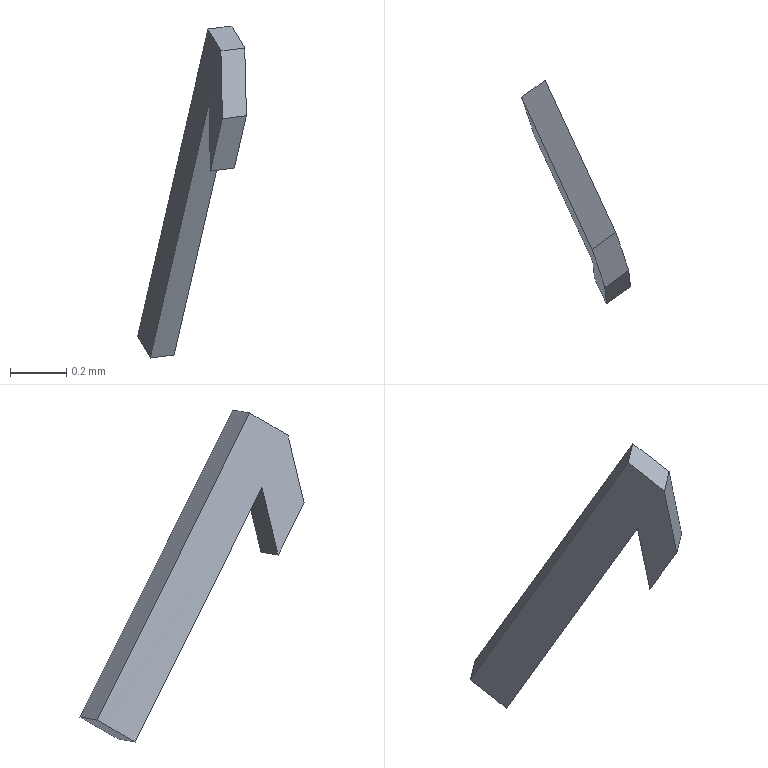Part | SolidWorks | features BaseBody 1 | 1 solid | 9 faces | box 0.3887 x 0.7999 x 1.186 mm | volume 0.02402 mm3 | plane 7 | cylinder 2 | commonest cylinder face diameters 16.8 x1 17 x1
STEP:
#1=CARTESIAN_POINT('',(1974.415,-240.873,992.396));
#2=VERTEX_POINT('',#1);
#3=CARTESIAN_POINT('',(1974.41,-240.816,992.638));
#4=VERTEX_POINT('',#3);
#5=CARTESIAN_POINT('',(1974.415,-240.873,992.396));
#6=CARTESIAN_POINT('',(1974.414,-240.854,992.476));
#7=CARTESIAN_POINT('',(1974.412,-240.835,992.557));
#8=CARTESIAN_POINT('',(1974.41,-240.816,992.638));
#9=B_SPLINE_CURVE_WITH_KNOTS('',3,(#5,#6,#7,#8),.UNSPECIFIED.,.F.,.F.,(4,4),(0.,1.),.UNSPECIFIED.);
#10=EDGE_CURVE('',#2,#4,#9,.T.);
#11=ORIENTED_EDGE('',*,*,#10,.T.);
#12=CARTESIAN_POINT('',(1974.364,-240.679,992.716));
#13=VERTEX_POINT('',#12);
#14=CARTESIAN_POINT('',(1966.499,-243.608,993.067));
#15=DIRECTION('',(0.2015,-0.436,0.8771));
#16=DIRECTION('',(-0.7309,-0.6631,-0.1618));
#17=AXIS2_PLACEMENT_3D('',#14,#15,#16);
#18=CIRCLE('',#17,8.4);
#19=EDGE_CURVE('',#4,#13,#18,.T.);
#20=ORIENTED_EDGE('',*,*,#19,.T.);
#21=CARTESIAN_POINT('',(1974.112,-240.134,991.62));
#22=VERTEX_POINT('',#21);
#23=CARTESIAN_POINT('',(1975.315,-242.737,996.856));
#24=DIRECTION('',(-0.2015,0.436,-0.8771));
#25=VECTOR('',#24,1000.);
#26=LINE('',#23,#25);
#27=EDGE_CURVE('',#13,#22,#26,.T.);
#28=ORIENTED_EDGE('',*,*,#27,.T.);
#29=CARTESIAN_POINT('',(1974.158,-240.271,991.541));
#30=VERTEX_POINT('',#29);
#31=CARTESIAN_POINT('',(1966.247,-243.063,991.97));
#32=DIRECTION('',(-0.2015,0.436,-0.8771));
#33=DIRECTION('',(-0.7309,-0.6631,-0.1618));
#34=AXIS2_PLACEMENT_3D('',#31,#32,#33);
#35=CIRCLE('',#34,8.4);
#36=EDGE_CURVE('',#22,#30,#35,.T.);
#37=ORIENTED_EDGE('',*,*,#36,.T.);
#38=CARTESIAN_POINT('',(1974.367,-240.723,992.451));
#39=VERTEX_POINT('',#38);
#40=CARTESIAN_POINT('',(1975.361,-242.874,996.778));
#41=DIRECTION('',(0.2015,-0.436,0.8771));
#42=VECTOR('',#41,1000.);
#43=LINE('',#40,#42);
#44=EDGE_CURVE('',#30,#39,#43,.T.);
#45=ORIENTED_EDGE('',*,*,#44,.T.);
#46=CARTESIAN_POINT('',(1974.372,-240.781,992.209));
#47=VERTEX_POINT('',#46);
#48=CARTESIAN_POINT('',(1974.372,-240.781,992.209));
#49=CARTESIAN_POINT('',(1974.371,-240.761,992.29));
#50=CARTESIAN_POINT('',(1974.369,-240.742,992.37));
#51=CARTESIAN_POINT('',(1974.367,-240.723,992.451));
#52=B_SPLINE_CURVE_WITH_KNOTS('',3,(#48,#49,#50,#51),.UNSPECIFIED.,.F.,.F.,(4,4),(0.,1.),.UNSPECIFIED.);
#53=EDGE_CURVE('',#47,#39,#52,.T.);
#54=ORIENTED_EDGE('',*,*,#53,.F.);
#55=CARTESIAN_POINT('',(1975.404,-243.013,996.699));
#56=DIRECTION('',(0.2015,-0.436,0.8771));
#57=VECTOR('',#56,1000.);
#58=LINE('',#55,#57);
#59=EDGE_CURVE('',#47,#2,#58,.T.);
#60=ORIENTED_EDGE('',*,*,#59,.T.);
#61=EDGE_LOOP('',(#11,#20,#28,#37,#45,#54,#60));
#62=FACE_OUTER_BOUND('',#61,.T.);
#63=CARTESIAN_POINT('',(1967.45,-245.666,997.207));
#64=DIRECTION('',(0.2015,-0.436,0.8771));
#65=DIRECTION('',(-0.7309,-0.6631,-0.1618));
#66=AXIS2_PLACEMENT_3D('',#63,#64,#65);
#67=CYLINDRICAL_SURFACE('',#66,8.4);
#68=ADVANCED_FACE('',(#62),#67,.F.);
#69=CARTESIAN_POINT('',(1974.501,-240.812,992.406));
#70=VERTEX_POINT('',#69);
#71=CARTESIAN_POINT('',(1974.458,-240.843,992.401));
#72=DIRECTION('',(-0.8088,-0.5792,-0.1022));
#73=VECTOR('',#72,1000.);
#74=LINE('',#71,#73);
#75=EDGE_CURVE('',#70,#2,#74,.T.);
#76=ORIENTED_EDGE('',*,*,#75,.T.);
#77=ORIENTED_EDGE('',*,*,#59,.F.);
#78=CARTESIAN_POINT('',(1974.458,-240.719,992.22));
#79=VERTEX_POINT('',#78);
#80=CARTESIAN_POINT('',(1974.415,-240.75,992.214));
#81=DIRECTION('',(-0.8088,-0.5792,-0.1022));
#82=VECTOR('',#81,1000.);
#83=LINE('',#80,#82);
#84=EDGE_CURVE('',#79,#47,#83,.T.);
#85=ORIENTED_EDGE('',*,*,#84,.F.);
#86=CARTESIAN_POINT('',(1974.48,-240.766,992.313));
#87=DIRECTION('',(0.2015,-0.436,0.8771));
#88=VECTOR('',#87,1000.);
#89=LINE('',#86,#88);
#90=EDGE_CURVE('',#79,#70,#89,.T.);
#91=ORIENTED_EDGE('',*,*,#90,.T.);
#92=EDGE_LOOP('',(#76,#77,#85,#91));
#93=FACE_OUTER_BOUND('',#92,.T.);
#94=CARTESIAN_POINT('',(1980.1,-236.679,992.933));
#95=DIRECTION('',(0.5526,-0.6888,-0.4693));
#96=DIRECTION('',(-0.2015,0.436,-0.8771));
#97=AXIS2_PLACEMENT_3D('',#94,#95,#96);
#98=PLANE('',#97);
#99=ADVANCED_FACE('',(#93),#98,.T.);
#100=ORIENTED_EDGE('',*,*,#84,.T.);
#101=ORIENTED_EDGE('',*,*,#53,.T.);
#102=CARTESIAN_POINT('',(1974.452,-240.662,992.462));
#103=VERTEX_POINT('',#102);
#104=CARTESIAN_POINT('',(1974.41,-240.693,992.456));
#105=DIRECTION('',(-0.8088,-0.5792,-0.1022));
#106=VECTOR('',#105,1000.);
#107=LINE('',#104,#106);
#108=EDGE_CURVE('',#103,#39,#107,.T.);
#109=ORIENTED_EDGE('',*,*,#108,.F.);
#110=CARTESIAN_POINT('',(1974.458,-240.719,992.22));
#111=CARTESIAN_POINT('',(1974.457,-240.708,992.268));
#112=CARTESIAN_POINT('',(1974.456,-240.696,992.317));
#113=CARTESIAN_POINT('',(1974.455,-240.685,992.365));
#114=CARTESIAN_POINT('',(1974.454,-240.673,992.413));
#115=CARTESIAN_POINT('',(1974.452,-240.662,992.462));
#116=B_SPLINE_CURVE_WITH_KNOTS('',5,(#110,#111,#112,#113,#114,#115),.UNSPECIFIED.,.F.,.F.,(6,6),(0.,1.),.UNSPECIFIED.);
#117=EDGE_CURVE('',#79,#103,#116,.T.);
#118=ORIENTED_EDGE('',*,*,#117,.F.);
#119=EDGE_LOOP('',(#100,#101,#109,#118));
#120=FACE_OUTER_BOUND('',#119,.T.);
#121=CARTESIAN_POINT('',(1980.051,-236.652,993.169));
#122=DIRECTION('',(-0.5528,0.8079,-0.2044));
#123=DIRECTION('',(-0.2009,0.1088,0.9736));
#124=AXIS2_PLACEMENT_3D('',#121,#122,#123);
#125=PLANE('',#124);
#126=ADVANCED_FACE('',(#120),#125,.T.);
#127=ORIENTED_EDGE('',*,*,#108,.T.);
#128=ORIENTED_EDGE('',*,*,#44,.F.);
#129=CARTESIAN_POINT('',(1974.243,-240.21,991.552));
#130=VERTEX_POINT('',#129);
#131=CARTESIAN_POINT('',(1974.201,-240.24,991.547));
#132=DIRECTION('',(-0.8088,-0.5792,-0.1022));
#133=VECTOR('',#132,1000.);
#134=LINE('',#131,#133);
#135=EDGE_CURVE('',#130,#30,#134,.T.);
#136=ORIENTED_EDGE('',*,*,#135,.F.);
#137=CARTESIAN_POINT('',(1974.348,-240.436,992.007));
#138=DIRECTION('',(0.2015,-0.436,0.8771));
#139=VECTOR('',#138,1000.);
#140=LINE('',#137,#139);
#141=EDGE_CURVE('',#130,#103,#140,.T.);
#142=ORIENTED_EDGE('',*,*,#141,.T.);
#143=EDGE_LOOP('',(#127,#128,#136,#142));
#144=FACE_OUTER_BOUND('',#143,.T.);
#145=CARTESIAN_POINT('',(1979.843,-236.2,992.259));
#146=DIRECTION('',(0.5526,-0.6888,-0.4693));
#147=DIRECTION('',(-0.2015,0.436,-0.8771));
#148=AXIS2_PLACEMENT_3D('',#145,#146,#147);
#149=PLANE('',#148);
#150=ADVANCED_FACE('',(#144),#149,.T.);
#151=ORIENTED_EDGE('',*,*,#135,.T.);
#152=ORIENTED_EDGE('',*,*,#36,.F.);
#153=CARTESIAN_POINT('',(1974.197,-240.074,991.63));
#154=VERTEX_POINT('',#153);
#155=CARTESIAN_POINT('',(1974.155,-240.104,991.625));
#156=DIRECTION('',(-0.8088,-0.5792,-0.1022));
#157=VECTOR('',#156,1000.);
#158=LINE('',#155,#157);
#159=EDGE_CURVE('',#154,#22,#158,.T.);
#160=ORIENTED_EDGE('',*,*,#159,.F.);
#161=CARTESIAN_POINT('',(1966.247,-243.063,991.97));
#162=DIRECTION('',(-0.2015,0.436,-0.8771));
#163=DIRECTION('',(-0.7309,-0.6631,-0.1618));
#164=AXIS2_PLACEMENT_3D('',#161,#162,#163);
#165=CIRCLE('',#164,8.5);
#166=EDGE_CURVE('',#154,#130,#165,.T.);
#167=ORIENTED_EDGE('',*,*,#166,.T.);
#168=EDGE_LOOP('',(#151,#152,#160,#167));
#169=FACE_OUTER_BOUND('',#168,.T.);
#170=CARTESIAN_POINT('',(1981.656,-238.46,990.719));
#171=DIRECTION('',(-0.2015,0.436,-0.8771));
#172=DIRECTION('',(-0.5526,0.6888,0.4693));
#173=AXIS2_PLACEMENT_3D('',#170,#171,#172);
#174=PLANE('',#173);
#175=ADVANCED_FACE('',(#169),#174,.T.);
#176=ORIENTED_EDGE('',*,*,#159,.T.);
#177=ORIENTED_EDGE('',*,*,#27,.F.);
#178=CARTESIAN_POINT('',(1974.449,-240.619,992.727));
#179=VERTEX_POINT('',#178);
#180=CARTESIAN_POINT('',(1974.406,-240.649,992.721));
#181=DIRECTION('',(-0.8088,-0.5792,-0.1022));
#182=VECTOR('',#181,1000.);
#183=LINE('',#180,#182);
#184=EDGE_CURVE('',#179,#13,#183,.T.);
#185=ORIENTED_EDGE('',*,*,#184,.F.);
#186=CARTESIAN_POINT('',(1974.323,-240.346,992.179));
#187=DIRECTION('',(-0.2015,0.436,-0.8771));
#188=VECTOR('',#187,1000.);
#189=LINE('',#186,#188);
#190=EDGE_CURVE('',#179,#154,#189,.T.);
#191=ORIENTED_EDGE('',*,*,#190,.T.);
#192=EDGE_LOOP('',(#176,#177,#185,#191));
#193=FACE_OUTER_BOUND('',#192,.T.);
#194=CARTESIAN_POINT('',(1980.008,-236.637,993.429));
#195=DIRECTION('',(-0.5526,0.6888,0.4693));
#196=DIRECTION('',(0.2015,-0.436,0.8771));
#197=AXIS2_PLACEMENT_3D('',#194,#195,#196);
#198=PLANE('',#197);
#199=ADVANCED_FACE('',(#193),#198,.T.);
#200=ORIENTED_EDGE('',*,*,#184,.T.);
#201=ORIENTED_EDGE('',*,*,#19,.F.);
#202=CARTESIAN_POINT('',(1974.495,-240.755,992.648));
#203=VERTEX_POINT('',#202);
#204=CARTESIAN_POINT('',(1974.452,-240.785,992.643));
#205=DIRECTION('',(-0.8088,-0.5792,-0.1022));
#206=VECTOR('',#205,1000.);
#207=LINE('',#204,#206);
#208=EDGE_CURVE('',#203,#4,#207,.T.);
#209=ORIENTED_EDGE('',*,*,#208,.F.);
#210=CARTESIAN_POINT('',(1966.499,-243.608,993.067));
#211=DIRECTION('',(0.2015,-0.436,0.8771));
#212=DIRECTION('',(-0.7309,-0.6631,-0.1618));
#213=AXIS2_PLACEMENT_3D('',#210,#211,#212);
#214=CIRCLE('',#213,8.5);
#215=EDGE_CURVE('',#203,#179,#214,.T.);
#216=ORIENTED_EDGE('',*,*,#215,.T.);
#217=EDGE_LOOP('',(#200,#201,#209,#216));
#218=FACE_OUTER_BOUND('',#217,.T.);
#219=CARTESIAN_POINT('',(1982.253,-239.435,991.522));
#220=DIRECTION('',(0.2015,-0.436,0.8771));
#221=DIRECTION('',(0.5526,-0.6888,-0.4693));
#222=AXIS2_PLACEMENT_3D('',#219,#220,#221);
#223=PLANE('',#222);
#224=ADVANCED_FACE('',(#218),#223,.T.);
#225=ORIENTED_EDGE('',*,*,#208,.T.);
#226=ORIENTED_EDGE('',*,*,#10,.F.);
#227=ORIENTED_EDGE('',*,*,#75,.F.);
#228=CARTESIAN_POINT('',(1974.501,-240.812,992.406));
#229=CARTESIAN_POINT('',(1974.5,-240.8,992.455));
#230=CARTESIAN_POINT('',(1974.499,-240.789,992.503));
#231=CARTESIAN_POINT('',(1974.498,-240.778,992.552));
#232=CARTESIAN_POINT('',(1974.496,-240.766,992.6));
#233=CARTESIAN_POINT('',(1974.495,-240.755,992.648));
#234=B_SPLINE_CURVE_WITH_KNOTS('',5,(#228,#229,#230,#231,#232,#233),.UNSPECIFIED.,.F.,.F.,(6,6),(0.,1.),.UNSPECIFIED.);
#235=EDGE_CURVE('',#70,#203,#234,.T.);
#236=ORIENTED_EDGE('',*,*,#235,.T.);
#237=EDGE_LOOP('',(#225,#226,#227,#236));
#238=FACE_OUTER_BOUND('',#237,.T.);
#239=CARTESIAN_POINT('',(1980.143,-236.771,993.119));
#240=DIRECTION('',(0.5528,-0.8079,0.2044));
#241=DIRECTION('',(0.2009,-0.1088,-0.9736));
#242=AXIS2_PLACEMENT_3D('',#239,#240,#241);
#243=PLANE('',#242);
#244=ADVANCED_FACE('',(#238),#243,.T.);
#245=ORIENTED_EDGE('',*,*,#90,.F.);
#246=ORIENTED_EDGE('',*,*,#117,.T.);
#247=ORIENTED_EDGE('',*,*,#141,.F.);
#248=ORIENTED_EDGE('',*,*,#166,.F.);
#249=ORIENTED_EDGE('',*,*,#190,.F.);
#250=ORIENTED_EDGE('',*,*,#215,.F.);
#251=ORIENTED_EDGE('',*,*,#235,.F.);
#252=EDGE_LOOP('',(#245,#246,#247,#248,#249,#250,#251));
#253=FACE_OUTER_BOUND('',#252,.T.);
#254=CARTESIAN_POINT('',(1967.45,-245.666,997.207));
#255=DIRECTION('',(0.2015,-0.436,0.8771));
#256=DIRECTION('',(-0.7309,-0.6631,-0.1618));
#257=AXIS2_PLACEMENT_3D('',#254,#255,#256);
#258=CYLINDRICAL_SURFACE('',#257,8.5);
#259=ADVANCED_FACE('',(#253),#258,.T.);
#260=CLOSED_SHELL('',(#68,#99,#126,#150,#175,#199,#224,#244,#259));
#261=MANIFOLD_SOLID_BREP('',#260);
#262=CARTESIAN_POINT('',(0.,0.,0.));
#263=DIRECTION('',(0.,0.,1.));
#264=DIRECTION('',(1.,0.,0.));
#265=AXIS2_PLACEMENT_3D('',#262,#263,#264);
#266=(LENGTH_UNIT()NAMED_UNIT(*)SI_UNIT(.MILLI.,.METRE.));
#267=UNCERTAINTY_MEASURE_WITH_UNIT(LENGTH_MEASURE(0.00001),#266,'','');
#268=(NAMED_UNIT(*)PLANE_ANGLE_UNIT()SI_UNIT($,.RADIAN.));
#269=(NAMED_UNIT(*)SI_UNIT($,.STERADIAN.)SOLID_ANGLE_UNIT());
#270=(GEOMETRIC_REPRESENTATION_CONTEXT(3)GLOBAL_UNCERTAINTY_ASSIGNED_CONTEXT((#267))GLOBAL_UNIT_ASSIGNED_CONTEXT((#266,#268,#269))REPRESENTATION_CONTEXT('',''));
#271=ADVANCED_BREP_SHAPE_REPRESENTATION('',(#261,#265),#270);